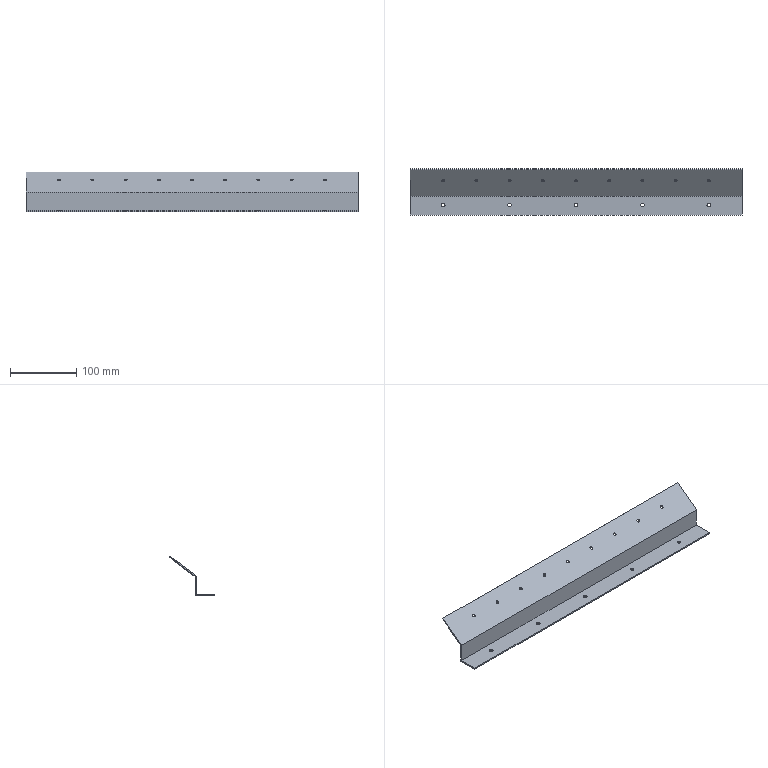Part | SolidWorks | features BaseBody 1 | 1 solid | 38 faces | box 500 x 69.2 x 60 mm | volume 106489 mm3 | cylinder 28 | plane 10 | commonest cylinder face diameters 4.4 x18 5.5 x10
STEP:
#1=CARTESIAN_POINT('',(546.946,-4176.013,1824.691));
#2=VERTEX_POINT('',#1);
#3=CARTESIAN_POINT('',(546.946,-4179.533,1822.051));
#4=VERTEX_POINT('',#3);
#5=CARTESIAN_POINT('',(546.946,-4177.773,1823.371));
#6=DIRECTION('',(0.,-0.6,0.8));
#7=DIRECTION('',(0.,-0.8,-0.6));
#8=AXIS2_PLACEMENT_3D('',#5,#6,#7);
#9=CIRCLE('',#8,2.2);
#10=EDGE_CURVE('',#2,#4,#9,.T.);
#11=ORIENTED_EDGE('',*,*,#10,.F.);
#12=CARTESIAN_POINT('',(546.946,-4177.213,1826.291));
#13=VERTEX_POINT('',#12);
#14=CARTESIAN_POINT('',(546.946,-4198.213,1854.291));
#15=DIRECTION('',(0.,-0.6,0.8));
#16=VECTOR('',#15,1000.);
#17=LINE('',#14,#16);
#18=EDGE_CURVE('',#2,#13,#17,.T.);
#19=ORIENTED_EDGE('',*,*,#18,.T.);
#20=CARTESIAN_POINT('',(546.946,-4180.733,1823.651));
#21=VERTEX_POINT('',#20);
#22=CARTESIAN_POINT('',(546.946,-4178.973,1824.971));
#23=DIRECTION('',(0.,0.6,-0.8));
#24=DIRECTION('',(0.,-0.8,-0.6));
#25=AXIS2_PLACEMENT_3D('',#22,#23,#24);
#26=CIRCLE('',#25,2.2);
#27=EDGE_CURVE('',#21,#13,#26,.T.);
#28=ORIENTED_EDGE('',*,*,#27,.F.);
#29=CARTESIAN_POINT('',(546.946,-4201.733,1851.651));
#30=DIRECTION('',(0.,-0.6,0.8));
#31=VECTOR('',#30,1000.);
#32=LINE('',#29,#31);
#33=EDGE_CURVE('',#4,#21,#32,.T.);
#34=ORIENTED_EDGE('',*,*,#33,.F.);
#35=EDGE_LOOP('',(#11,#19,#28,#34));
#36=FACE_OUTER_BOUND('',#35,.T.);
#37=CARTESIAN_POINT('',(546.946,-4199.973,1852.971));
#38=DIRECTION('',(0.,-0.6,0.8));
#39=DIRECTION('',(0.,-0.8,-0.6));
#40=AXIS2_PLACEMENT_3D('',#37,#38,#39);
#41=CYLINDRICAL_SURFACE('',#40,2.2);
#42=ADVANCED_FACE('',(#36),#41,.F.);
#43=CARTESIAN_POINT('',(446.946,-4176.013,1824.691));
#44=VERTEX_POINT('',#43);
#45=CARTESIAN_POINT('',(446.946,-4179.533,1822.051));
#46=VERTEX_POINT('',#45);
#47=CARTESIAN_POINT('',(446.946,-4177.773,1823.371));
#48=DIRECTION('',(0.,-0.6,0.8));
#49=DIRECTION('',(0.,-0.8,-0.6));
#50=AXIS2_PLACEMENT_3D('',#47,#48,#49);
#51=CIRCLE('',#50,2.2);
#52=EDGE_CURVE('',#44,#46,#51,.T.);
#53=ORIENTED_EDGE('',*,*,#52,.F.);
#54=CARTESIAN_POINT('',(446.946,-4177.213,1826.291));
#55=VERTEX_POINT('',#54);
#56=CARTESIAN_POINT('',(446.946,-4198.213,1854.291));
#57=DIRECTION('',(0.,-0.6,0.8));
#58=VECTOR('',#57,1000.);
#59=LINE('',#56,#58);
#60=EDGE_CURVE('',#44,#55,#59,.T.);
#61=ORIENTED_EDGE('',*,*,#60,.T.);
#62=CARTESIAN_POINT('',(446.946,-4180.733,1823.651));
#63=VERTEX_POINT('',#62);
#64=CARTESIAN_POINT('',(446.946,-4178.973,1824.971));
#65=DIRECTION('',(0.,0.6,-0.8));
#66=DIRECTION('',(0.,-0.8,-0.6));
#67=AXIS2_PLACEMENT_3D('',#64,#65,#66);
#68=CIRCLE('',#67,2.2);
#69=EDGE_CURVE('',#63,#55,#68,.T.);
#70=ORIENTED_EDGE('',*,*,#69,.F.);
#71=CARTESIAN_POINT('',(446.946,-4201.733,1851.651));
#72=DIRECTION('',(0.,-0.6,0.8));
#73=VECTOR('',#72,1000.);
#74=LINE('',#71,#73);
#75=EDGE_CURVE('',#46,#63,#74,.T.);
#76=ORIENTED_EDGE('',*,*,#75,.F.);
#77=EDGE_LOOP('',(#53,#61,#70,#76));
#78=FACE_OUTER_BOUND('',#77,.T.);
#79=CARTESIAN_POINT('',(446.946,-4199.973,1852.971));
#80=DIRECTION('',(0.,-0.6,0.8));
#81=DIRECTION('',(0.,-0.8,-0.6));
#82=AXIS2_PLACEMENT_3D('',#79,#80,#81);
#83=CYLINDRICAL_SURFACE('',#82,2.2);
#84=ADVANCED_FACE('',(#78),#83,.F.);
#85=CARTESIAN_POINT('',(346.946,-4176.013,1824.691));
#86=VERTEX_POINT('',#85);
#87=CARTESIAN_POINT('',(346.946,-4179.533,1822.051));
#88=VERTEX_POINT('',#87);
#89=CARTESIAN_POINT('',(346.946,-4177.773,1823.371));
#90=DIRECTION('',(0.,-0.6,0.8));
#91=DIRECTION('',(0.,-0.8,-0.6));
#92=AXIS2_PLACEMENT_3D('',#89,#90,#91);
#93=CIRCLE('',#92,2.2);
#94=EDGE_CURVE('',#86,#88,#93,.T.);
#95=ORIENTED_EDGE('',*,*,#94,.F.);
#96=CARTESIAN_POINT('',(346.946,-4177.213,1826.291));
#97=VERTEX_POINT('',#96);
#98=CARTESIAN_POINT('',(346.946,-4198.213,1854.291));
#99=DIRECTION('',(0.,-0.6,0.8));
#100=VECTOR('',#99,1000.);
#101=LINE('',#98,#100);
#102=EDGE_CURVE('',#86,#97,#101,.T.);
#103=ORIENTED_EDGE('',*,*,#102,.T.);
#104=CARTESIAN_POINT('',(346.946,-4180.733,1823.651));
#105=VERTEX_POINT('',#104);
#106=CARTESIAN_POINT('',(346.946,-4178.973,1824.971));
#107=DIRECTION('',(0.,0.6,-0.8));
#108=DIRECTION('',(0.,-0.8,-0.6));
#109=AXIS2_PLACEMENT_3D('',#106,#107,#108);
#110=CIRCLE('',#109,2.2);
#111=EDGE_CURVE('',#105,#97,#110,.T.);
#112=ORIENTED_EDGE('',*,*,#111,.F.);
#113=CARTESIAN_POINT('',(346.946,-4201.733,1851.651));
#114=DIRECTION('',(0.,-0.6,0.8));
#115=VECTOR('',#114,1000.);
#116=LINE('',#113,#115);
#117=EDGE_CURVE('',#88,#105,#116,.T.);
#118=ORIENTED_EDGE('',*,*,#117,.F.);
#119=EDGE_LOOP('',(#95,#103,#112,#118));
#120=FACE_OUTER_BOUND('',#119,.T.);
#121=CARTESIAN_POINT('',(346.946,-4199.973,1852.971));
#122=DIRECTION('',(0.,-0.6,0.8));
#123=DIRECTION('',(0.,-0.8,-0.6));
#124=AXIS2_PLACEMENT_3D('',#121,#122,#123);
#125=CYLINDRICAL_SURFACE('',#124,2.2);
#126=ADVANCED_FACE('',(#120),#125,.F.);
#127=CARTESIAN_POINT('',(646.946,-4176.013,1824.691));
#128=VERTEX_POINT('',#127);
#129=CARTESIAN_POINT('',(646.946,-4179.533,1822.051));
#130=VERTEX_POINT('',#129);
#131=CARTESIAN_POINT('',(646.946,-4177.773,1823.371));
#132=DIRECTION('',(0.,-0.6,0.8));
#133=DIRECTION('',(0.,-0.8,-0.6));
#134=AXIS2_PLACEMENT_3D('',#131,#132,#133);
#135=CIRCLE('',#134,2.2);
#136=EDGE_CURVE('',#128,#130,#135,.T.);
#137=ORIENTED_EDGE('',*,*,#136,.F.);
#138=CARTESIAN_POINT('',(646.946,-4177.213,1826.291));
#139=VERTEX_POINT('',#138);
#140=CARTESIAN_POINT('',(646.946,-4198.213,1854.291));
#141=DIRECTION('',(0.,-0.6,0.8));
#142=VECTOR('',#141,1000.);
#143=LINE('',#140,#142);
#144=EDGE_CURVE('',#128,#139,#143,.T.);
#145=ORIENTED_EDGE('',*,*,#144,.T.);
#146=CARTESIAN_POINT('',(646.946,-4180.733,1823.651));
#147=VERTEX_POINT('',#146);
#148=CARTESIAN_POINT('',(646.946,-4178.973,1824.971));
#149=DIRECTION('',(0.,0.6,-0.8));
#150=DIRECTION('',(0.,-0.8,-0.6));
#151=AXIS2_PLACEMENT_3D('',#148,#149,#150);
#152=CIRCLE('',#151,2.2);
#153=EDGE_CURVE('',#147,#139,#152,.T.);
#154=ORIENTED_EDGE('',*,*,#153,.F.);
#155=CARTESIAN_POINT('',(646.946,-4201.733,1851.651));
#156=DIRECTION('',(0.,-0.6,0.8));
#157=VECTOR('',#156,1000.);
#158=LINE('',#155,#157);
#159=EDGE_CURVE('',#130,#147,#158,.T.);
#160=ORIENTED_EDGE('',*,*,#159,.F.);
#161=EDGE_LOOP('',(#137,#145,#154,#160));
#162=FACE_OUTER_BOUND('',#161,.T.);
#163=CARTESIAN_POINT('',(646.946,-4199.973,1852.971));
#164=DIRECTION('',(0.,-0.6,0.8));
#165=DIRECTION('',(0.,-0.8,-0.6));
#166=AXIS2_PLACEMENT_3D('',#163,#164,#165);
#167=CYLINDRICAL_SURFACE('',#166,2.2);
#168=ADVANCED_FACE('',(#162),#167,.F.);
#169=CARTESIAN_POINT('',(746.946,-4176.013,1824.691));
#170=VERTEX_POINT('',#169);
#171=CARTESIAN_POINT('',(746.946,-4179.533,1822.051));
#172=VERTEX_POINT('',#171);
#173=CARTESIAN_POINT('',(746.946,-4177.773,1823.371));
#174=DIRECTION('',(0.,-0.6,0.8));
#175=DIRECTION('',(0.,-0.8,-0.6));
#176=AXIS2_PLACEMENT_3D('',#173,#174,#175);
#177=CIRCLE('',#176,2.2);
#178=EDGE_CURVE('',#170,#172,#177,.T.);
#179=ORIENTED_EDGE('',*,*,#178,.F.);
#180=CARTESIAN_POINT('',(746.946,-4177.213,1826.291));
#181=VERTEX_POINT('',#180);
#182=CARTESIAN_POINT('',(746.946,-4198.213,1854.291));
#183=DIRECTION('',(0.,-0.6,0.8));
#184=VECTOR('',#183,1000.);
#185=LINE('',#182,#184);
#186=EDGE_CURVE('',#170,#181,#185,.T.);
#187=ORIENTED_EDGE('',*,*,#186,.T.);
#188=CARTESIAN_POINT('',(746.946,-4180.733,1823.651));
#189=VERTEX_POINT('',#188);
#190=CARTESIAN_POINT('',(746.946,-4178.973,1824.971));
#191=DIRECTION('',(0.,0.6,-0.8));
#192=DIRECTION('',(0.,-0.8,-0.6));
#193=AXIS2_PLACEMENT_3D('',#190,#191,#192);
#194=CIRCLE('',#193,2.2);
#195=EDGE_CURVE('',#189,#181,#194,.T.);
#196=ORIENTED_EDGE('',*,*,#195,.F.);
#197=CARTESIAN_POINT('',(746.946,-4201.733,1851.651));
#198=DIRECTION('',(0.,-0.6,0.8));
#199=VECTOR('',#198,1000.);
#200=LINE('',#197,#199);
#201=EDGE_CURVE('',#172,#189,#200,.T.);
#202=ORIENTED_EDGE('',*,*,#201,.F.);
#203=EDGE_LOOP('',(#179,#187,#196,#202));
#204=FACE_OUTER_BOUND('',#203,.T.);
#205=CARTESIAN_POINT('',(746.946,-4199.973,1852.971));
#206=DIRECTION('',(0.,-0.6,0.8));
#207=DIRECTION('',(0.,-0.8,-0.6));
#208=AXIS2_PLACEMENT_3D('',#205,#206,#207);
#209=CYLINDRICAL_SURFACE('',#208,2.2);
#210=ADVANCED_FACE('',(#204),#209,.F.);
#211=CARTESIAN_POINT('',(596.946,-4176.013,1824.691));
#212=VERTEX_POINT('',#211);
#213=CARTESIAN_POINT('',(596.946,-4179.533,1822.051));
#214=VERTEX_POINT('',#213);
#215=CARTESIAN_POINT('',(596.946,-4177.773,1823.371));
#216=DIRECTION('',(0.,-0.6,0.8));
#217=DIRECTION('',(0.,-0.8,-0.6));
#218=AXIS2_PLACEMENT_3D('',#215,#216,#217);
#219=CIRCLE('',#218,2.2);
#220=EDGE_CURVE('',#212,#214,#219,.T.);
#221=ORIENTED_EDGE('',*,*,#220,.F.);
#222=CARTESIAN_POINT('',(596.946,-4177.213,1826.291));
#223=VERTEX_POINT('',#222);
#224=CARTESIAN_POINT('',(596.946,-4198.213,1854.291));
#225=DIRECTION('',(0.,-0.6,0.8));
#226=VECTOR('',#225,1000.);
#227=LINE('',#224,#226);
#228=EDGE_CURVE('',#212,#223,#227,.T.);
#229=ORIENTED_EDGE('',*,*,#228,.T.);
#230=CARTESIAN_POINT('',(596.946,-4180.733,1823.651));
#231=VERTEX_POINT('',#230);
#232=CARTESIAN_POINT('',(596.946,-4178.973,1824.971));
#233=DIRECTION('',(0.,0.6,-0.8));
#234=DIRECTION('',(0.,-0.8,-0.6));
#235=AXIS2_PLACEMENT_3D('',#232,#233,#234);
#236=CIRCLE('',#235,2.2);
#237=EDGE_CURVE('',#231,#223,#236,.T.);
#238=ORIENTED_EDGE('',*,*,#237,.F.);
#239=CARTESIAN_POINT('',(596.946,-4201.733,1851.651));
#240=DIRECTION('',(0.,-0.6,0.8));
#241=VECTOR('',#240,1000.);
#242=LINE('',#239,#241);
#243=EDGE_CURVE('',#214,#231,#242,.T.);
#244=ORIENTED_EDGE('',*,*,#243,.F.);
#245=EDGE_LOOP('',(#221,#229,#238,#244));
#246=FACE_OUTER_BOUND('',#245,.T.);
#247=CARTESIAN_POINT('',(596.946,-4199.973,1852.971));
#248=DIRECTION('',(0.,-0.6,0.8));
#249=DIRECTION('',(0.,-0.8,-0.6));
#250=AXIS2_PLACEMENT_3D('',#247,#248,#249);
#251=CYLINDRICAL_SURFACE('',#250,2.2);
#252=ADVANCED_FACE('',(#246),#251,.F.);
#253=CARTESIAN_POINT('',(696.946,-4176.013,1824.691));
#254=VERTEX_POINT('',#253);
#255=CARTESIAN_POINT('',(696.946,-4179.533,1822.051));
#256=VERTEX_POINT('',#255);
#257=CARTESIAN_POINT('',(696.946,-4177.773,1823.371));
#258=DIRECTION('',(0.,-0.6,0.8));
#259=DIRECTION('',(0.,-0.8,-0.6));
#260=AXIS2_PLACEMENT_3D('',#257,#258,#259);
#261=CIRCLE('',#260,2.2);
#262=EDGE_CURVE('',#254,#256,#261,.T.);
#263=ORIENTED_EDGE('',*,*,#262,.F.);
#264=CARTESIAN_POINT('',(696.946,-4177.213,1826.291));
#265=VERTEX_POINT('',#264);
#266=CARTESIAN_POINT('',(696.946,-4198.213,1854.291));
#267=DIRECTION('',(0.,-0.6,0.8));
#268=VECTOR('',#267,1000.);
#269=LINE('',#266,#268);
#270=EDGE_CURVE('',#254,#265,#269,.T.);
#271=ORIENTED_EDGE('',*,*,#270,.T.);
#272=CARTESIAN_POINT('',(696.946,-4180.733,1823.651));
#273=VERTEX_POINT('',#272);
#274=CARTESIAN_POINT('',(696.946,-4178.973,1824.971));
#275=DIRECTION('',(0.,0.6,-0.8));
#276=DIRECTION('',(0.,-0.8,-0.6));
#277=AXIS2_PLACEMENT_3D('',#274,#275,#276);
#278=CIRCLE('',#277,2.2);
#279=EDGE_CURVE('',#273,#265,#278,.T.);
#280=ORIENTED_EDGE('',*,*,#279,.F.);
#281=CARTESIAN_POINT('',(696.946,-4201.733,1851.651));
#282=DIRECTION('',(0.,-0.6,0.8));
#283=VECTOR('',#282,1000.);
#284=LINE('',#281,#283);
#285=EDGE_CURVE('',#256,#273,#284,.T.);
#286=ORIENTED_EDGE('',*,*,#285,.F.);
#287=EDGE_LOOP('',(#263,#271,#280,#286));
#288=FACE_OUTER_BOUND('',#287,.T.);
#289=CARTESIAN_POINT('',(696.946,-4199.973,1852.971));
#290=DIRECTION('',(0.,-0.6,0.8));
#291=DIRECTION('',(0.,-0.8,-0.6));
#292=AXIS2_PLACEMENT_3D('',#289,#290,#291);
#293=CYLINDRICAL_SURFACE('',#292,2.2);
#294=ADVANCED_FACE('',(#288),#293,.F.);
#295=CARTESIAN_POINT('',(396.946,-4176.013,1824.691));
#296=VERTEX_POINT('',#295);
#297=CARTESIAN_POINT('',(396.946,-4179.533,1822.051));
#298=VERTEX_POINT('',#297);
#299=CARTESIAN_POINT('',(396.946,-4177.773,1823.371));
#300=DIRECTION('',(0.,-0.6,0.8));
#301=DIRECTION('',(0.,-0.8,-0.6));
#302=AXIS2_PLACEMENT_3D('',#299,#300,#301);
#303=CIRCLE('',#302,2.2);
#304=EDGE_CURVE('',#296,#298,#303,.T.);
#305=ORIENTED_EDGE('',*,*,#304,.F.);
#306=CARTESIAN_POINT('',(396.946,-4177.213,1826.291));
#307=VERTEX_POINT('',#306);
#308=CARTESIAN_POINT('',(396.946,-4198.213,1854.291));
#309=DIRECTION('',(0.,-0.6,0.8));
#310=VECTOR('',#309,1000.);
#311=LINE('',#308,#310);
#312=EDGE_CURVE('',#296,#307,#311,.T.);
#313=ORIENTED_EDGE('',*,*,#312,.T.);
#314=CARTESIAN_POINT('',(396.946,-4180.733,1823.651));
#315=VERTEX_POINT('',#314);
#316=CARTESIAN_POINT('',(396.946,-4178.973,1824.971));
#317=DIRECTION('',(0.,0.6,-0.8));
#318=DIRECTION('',(0.,-0.8,-0.6));
#319=AXIS2_PLACEMENT_3D('',#316,#317,#318);
#320=CIRCLE('',#319,2.2);
#321=EDGE_CURVE('',#315,#307,#320,.T.);
#322=ORIENTED_EDGE('',*,*,#321,.F.);
#323=CARTESIAN_POINT('',(396.946,-4201.733,1851.651));
#324=DIRECTION('',(0.,-0.6,0.8));
#325=VECTOR('',#324,1000.);
#326=LINE('',#323,#325);
#327=EDGE_CURVE('',#298,#315,#326,.T.);
#328=ORIENTED_EDGE('',*,*,#327,.F.);
#329=EDGE_LOOP('',(#305,#313,#322,#328));
#330=FACE_OUTER_BOUND('',#329,.T.);
#331=CARTESIAN_POINT('',(396.946,-4199.973,1852.971));
#332=DIRECTION('',(0.,-0.6,0.8));
#333=DIRECTION('',(0.,-0.8,-0.6));
#334=AXIS2_PLACEMENT_3D('',#331,#332,#333);
#335=CYLINDRICAL_SURFACE('',#334,2.2);
#336=ADVANCED_FACE('',(#330),#335,.F.);
#337=CARTESIAN_POINT('',(496.946,-4176.013,1824.691));
#338=VERTEX_POINT('',#337);
#339=CARTESIAN_POINT('',(496.946,-4179.533,1822.051));
#340=VERTEX_POINT('',#339);
#341=CARTESIAN_POINT('',(496.946,-4177.773,1823.371));
#342=DIRECTION('',(0.,-0.6,0.8));
#343=DIRECTION('',(0.,-0.8,-0.6));
#344=AXIS2_PLACEMENT_3D('',#341,#342,#343);
#345=CIRCLE('',#344,2.2);
#346=EDGE_CURVE('',#338,#340,#345,.T.);
#347=ORIENTED_EDGE('',*,*,#346,.F.);
#348=CARTESIAN_POINT('',(496.946,-4177.213,1826.291));
#349=VERTEX_POINT('',#348);
#350=CARTESIAN_POINT('',(496.946,-4198.213,1854.291));
#351=DIRECTION('',(0.,-0.6,0.8));
#352=VECTOR('',#351,1000.);
#353=LINE('',#350,#352);
#354=EDGE_CURVE('',#338,#349,#353,.T.);
#355=ORIENTED_EDGE('',*,*,#354,.T.);
#356=CARTESIAN_POINT('',(496.946,-4180.733,1823.651));
#357=VERTEX_POINT('',#356);
#358=CARTESIAN_POINT('',(496.946,-4178.973,1824.971));
#359=DIRECTION('',(0.,0.6,-0.8));
#360=DIRECTION('',(0.,-0.8,-0.6));
#361=AXIS2_PLACEMENT_3D('',#358,#359,#360);
#362=CIRCLE('',#361,2.2);
#363=EDGE_CURVE('',#357,#349,#362,.T.);
#364=ORIENTED_EDGE('',*,*,#363,.F.);
#365=CARTESIAN_POINT('',(496.946,-4201.733,1851.651));
#366=DIRECTION('',(0.,-0.6,0.8));
#367=VECTOR('',#366,1000.);
#368=LINE('',#365,#367);
#369=EDGE_CURVE('',#340,#357,#368,.T.);
#370=ORIENTED_EDGE('',*,*,#369,.F.);
#371=EDGE_LOOP('',(#347,#355,#364,#370));
#372=FACE_OUTER_BOUND('',#371,.T.);
#373=CARTESIAN_POINT('',(496.946,-4199.973,1852.971));
#374=DIRECTION('',(0.,-0.6,0.8));
#375=DIRECTION('',(0.,-0.8,-0.6));
#376=AXIS2_PLACEMENT_3D('',#373,#374,#375);
#377=CYLINDRICAL_SURFACE('',#376,2.2);
#378=ADVANCED_FACE('',(#372),#377,.F.);
#379=CARTESIAN_POINT('',(444.196,-4215.973,1776.971));
#380=VERTEX_POINT('',#379);
#381=CARTESIAN_POINT('',(449.696,-4215.973,1776.971));
#382=VERTEX_POINT('',#381);
#383=CARTESIAN_POINT('',(446.946,-4215.973,1776.971));
#384=DIRECTION('',(0.,0.,1.));
#385=DIRECTION('',(1.,0.,0.));
#386=AXIS2_PLACEMENT_3D('',#383,#384,#385);
#387=CIRCLE('',#386,2.75);
#388=EDGE_CURVE('',#380,#382,#387,.T.);
#389=ORIENTED_EDGE('',*,*,#388,.F.);
#390=CARTESIAN_POINT('',(444.196,-4215.973,1778.971));
#391=VERTEX_POINT('',#390);
#392=CARTESIAN_POINT('',(444.196,-4215.973,1778.308));
#393=DIRECTION('',(0.,0.,1.));
#394=VECTOR('',#393,1000.);
#395=LINE('',#392,#394);
#396=EDGE_CURVE('',#380,#391,#395,.T.);
#397=ORIENTED_EDGE('',*,*,#396,.T.);
#398=CARTESIAN_POINT('',(449.696,-4215.973,1778.971));
#399=VERTEX_POINT('',#398);
#400=CARTESIAN_POINT('',(446.946,-4215.973,1778.971));
#401=DIRECTION('',(0.,0.,-1.));
#402=DIRECTION('',(1.,0.,0.));
#403=AXIS2_PLACEMENT_3D('',#400,#401,#402);
#404=CIRCLE('',#403,2.75);
#405=EDGE_CURVE('',#399,#391,#404,.T.);
#406=ORIENTED_EDGE('',*,*,#405,.F.);
#407=CARTESIAN_POINT('',(449.696,-4215.973,1778.308));
#408=DIRECTION('',(0.,0.,1.));
#409=VECTOR('',#408,1000.);
#410=LINE('',#407,#409);
#411=EDGE_CURVE('',#382,#399,#410,.T.);
#412=ORIENTED_EDGE('',*,*,#411,.F.);
#413=EDGE_LOOP('',(#389,#397,#406,#412));
#414=FACE_OUTER_BOUND('',#413,.T.);
#415=CARTESIAN_POINT('',(446.946,-4215.973,1778.308));
#416=DIRECTION('',(0.,0.,1.));
#417=DIRECTION('',(1.,0.,0.));
#418=AXIS2_PLACEMENT_3D('',#415,#416,#417);
#419=CYLINDRICAL_SURFACE('',#418,2.75);
#420=ADVANCED_FACE('',(#414),#419,.F.);
#421=CARTESIAN_POINT('',(549.696,-4215.973,1778.971));
#422=VERTEX_POINT('',#421);
#423=CARTESIAN_POINT('',(544.196,-4215.973,1778.971));
#424=VERTEX_POINT('',#423);
#425=CARTESIAN_POINT('',(546.946,-4215.973,1778.971));
#426=DIRECTION('',(0.,0.,-1.));
#427=DIRECTION('',(-1.,0.,0.));
#428=AXIS2_PLACEMENT_3D('',#425,#426,#427);
#429=CIRCLE('',#428,2.75);
#430=EDGE_CURVE('',#422,#424,#429,.T.);
#431=ORIENTED_EDGE('',*,*,#430,.F.);
#432=CARTESIAN_POINT('',(549.696,-4215.973,1776.971));
#433=VERTEX_POINT('',#432);
#434=CARTESIAN_POINT('',(549.696,-4215.973,1778.308));
#435=DIRECTION('',(0.,0.,-1.));
#436=VECTOR('',#435,1000.);
#437=LINE('',#434,#436);
#438=EDGE_CURVE('',#422,#433,#437,.T.);
#439=ORIENTED_EDGE('',*,*,#438,.T.);
#440=CARTESIAN_POINT('',(544.196,-4215.973,1776.971));
#441=VERTEX_POINT('',#440);
#442=CARTESIAN_POINT('',(546.946,-4215.973,1776.971));
#443=DIRECTION('',(0.,0.,1.));
#444=DIRECTION('',(-1.,0.,0.));
#445=AXIS2_PLACEMENT_3D('',#442,#443,#444);
#446=CIRCLE('',#445,2.75);
#447=EDGE_CURVE('',#441,#433,#446,.T.);
#448=ORIENTED_EDGE('',*,*,#447,.F.);
#449=CARTESIAN_POINT('',(544.196,-4215.973,1778.308));
#450=DIRECTION('',(0.,0.,-1.));
#451=VECTOR('',#450,1000.);
#452=LINE('',#449,#451);
#453=EDGE_CURVE('',#424,#441,#452,.T.);
#454=ORIENTED_EDGE('',*,*,#453,.F.);
#455=EDGE_LOOP('',(#431,#439,#448,#454));
#456=FACE_OUTER_BOUND('',#455,.T.);
#457=CARTESIAN_POINT('',(546.946,-4215.973,1778.308));
#458=DIRECTION('',(0.,0.,-1.));
#459=DIRECTION('',(-1.,0.,0.));
#460=AXIS2_PLACEMENT_3D('',#457,#458,#459);
#461=CYLINDRICAL_SURFACE('',#460,2.75);
#462=ADVANCED_FACE('',(#456),#461,.F.);
#463=CARTESIAN_POINT('',(749.696,-4215.973,1778.971));
#464=VERTEX_POINT('',#463);
#465=CARTESIAN_POINT('',(744.196,-4215.973,1778.971));
#466=VERTEX_POINT('',#465);
#467=CARTESIAN_POINT('',(746.946,-4215.973,1778.971));
#468=DIRECTION('',(0.,0.,-1.));
#469=DIRECTION('',(-1.,0.,0.));
#470=AXIS2_PLACEMENT_3D('',#467,#468,#469);
#471=CIRCLE('',#470,2.75);
#472=EDGE_CURVE('',#464,#466,#471,.T.);
#473=ORIENTED_EDGE('',*,*,#472,.F.);
#474=CARTESIAN_POINT('',(749.696,-4215.973,1776.971));
#475=VERTEX_POINT('',#474);
#476=CARTESIAN_POINT('',(749.696,-4215.973,1778.308));
#477=DIRECTION('',(0.,0.,-1.));
#478=VECTOR('',#477,1000.);
#479=LINE('',#476,#478);
#480=EDGE_CURVE('',#464,#475,#479,.T.);
#481=ORIENTED_EDGE('',*,*,#480,.T.);
#482=CARTESIAN_POINT('',(744.196,-4215.973,1776.971));
#483=VERTEX_POINT('',#482);
#484=CARTESIAN_POINT('',(746.946,-4215.973,1776.971));
#485=DIRECTION('',(0.,0.,1.));
#486=DIRECTION('',(-1.,0.,0.));
#487=AXIS2_PLACEMENT_3D('',#484,#485,#486);
#488=CIRCLE('',#487,2.75);
#489=EDGE_CURVE('',#483,#475,#488,.T.);
#490=ORIENTED_EDGE('',*,*,#489,.F.);
#491=CARTESIAN_POINT('',(744.196,-4215.973,1778.308));
#492=DIRECTION('',(0.,0.,-1.));
#493=VECTOR('',#492,1000.);
#494=LINE('',#491,#493);
#495=EDGE_CURVE('',#466,#483,#494,.T.);
#496=ORIENTED_EDGE('',*,*,#495,.F.);
#497=EDGE_LOOP('',(#473,#481,#490,#496));
#498=FACE_OUTER_BOUND('',#497,.T.);
#499=CARTESIAN_POINT('',(746.946,-4215.973,1778.308));
#500=DIRECTION('',(0.,0.,-1.));
#501=DIRECTION('',(-1.,0.,0.));
#502=AXIS2_PLACEMENT_3D('',#499,#500,#501);
#503=CYLINDRICAL_SURFACE('',#502,2.75);
#504=ADVANCED_FACE('',(#498),#503,.F.);
#505=CARTESIAN_POINT('',(649.696,-4215.973,1778.971));
#506=VERTEX_POINT('',#505);
#507=CARTESIAN_POINT('',(644.196,-4215.973,1778.971));
#508=VERTEX_POINT('',#507);
#509=CARTESIAN_POINT('',(646.946,-4215.973,1778.971));
#510=DIRECTION('',(0.,0.,-1.));
#511=DIRECTION('',(-1.,0.,0.));
#512=AXIS2_PLACEMENT_3D('',#509,#510,#511);
#513=CIRCLE('',#512,2.75);
#514=EDGE_CURVE('',#506,#508,#513,.T.);
#515=ORIENTED_EDGE('',*,*,#514,.F.);
#516=CARTESIAN_POINT('',(649.696,-4215.973,1776.971));
#517=VERTEX_POINT('',#516);
#518=CARTESIAN_POINT('',(649.696,-4215.973,1778.308));
#519=DIRECTION('',(0.,0.,-1.));
#520=VECTOR('',#519,1000.);
#521=LINE('',#518,#520);
#522=EDGE_CURVE('',#506,#517,#521,.T.);
#523=ORIENTED_EDGE('',*,*,#522,.T.);
#524=CARTESIAN_POINT('',(644.196,-4215.973,1776.971));
#525=VERTEX_POINT('',#524);
#526=CARTESIAN_POINT('',(646.946,-4215.973,1776.971));
#527=DIRECTION('',(0.,0.,1.));
#528=DIRECTION('',(-1.,0.,0.));
#529=AXIS2_PLACEMENT_3D('',#526,#527,#528);
#530=CIRCLE('',#529,2.75);
#531=EDGE_CURVE('',#525,#517,#530,.T.);
#532=ORIENTED_EDGE('',*,*,#531,.F.);
#533=CARTESIAN_POINT('',(644.196,-4215.973,1778.308));
#534=DIRECTION('',(0.,0.,-1.));
#535=VECTOR('',#534,1000.);
#536=LINE('',#533,#535);
#537=EDGE_CURVE('',#508,#525,#536,.T.);
#538=ORIENTED_EDGE('',*,*,#537,.F.);
#539=EDGE_LOOP('',(#515,#523,#532,#538));
#540=FACE_OUTER_BOUND('',#539,.T.);
#541=CARTESIAN_POINT('',(646.946,-4215.973,1778.308));
#542=DIRECTION('',(0.,0.,-1.));
#543=DIRECTION('',(-1.,0.,0.));
#544=AXIS2_PLACEMENT_3D('',#541,#542,#543);
#545=CYLINDRICAL_SURFACE('',#544,2.75);
#546=ADVANCED_FACE('',(#540),#545,.F.);
#547=CARTESIAN_POINT('',(344.196,-4215.973,1776.971));
#548=VERTEX_POINT('',#547);
#549=CARTESIAN_POINT('',(349.696,-4215.973,1776.971));
#550=VERTEX_POINT('',#549);
#551=CARTESIAN_POINT('',(346.946,-4215.973,1776.971));
#552=DIRECTION('',(0.,0.,1.));
#553=DIRECTION('',(1.,0.,0.));
#554=AXIS2_PLACEMENT_3D('',#551,#552,#553);
#555=CIRCLE('',#554,2.75);
#556=EDGE_CURVE('',#548,#550,#555,.T.);
#557=ORIENTED_EDGE('',*,*,#556,.F.);
#558=CARTESIAN_POINT('',(344.196,-4215.973,1778.971));
#559=VERTEX_POINT('',#558);
#560=CARTESIAN_POINT('',(344.196,-4215.973,1778.308));
#561=DIRECTION('',(0.,0.,1.));
#562=VECTOR('',#561,1000.);
#563=LINE('',#560,#562);
#564=EDGE_CURVE('',#548,#559,#563,.T.);
#565=ORIENTED_EDGE('',*,*,#564,.T.);
#566=CARTESIAN_POINT('',(349.696,-4215.973,1778.971));
#567=VERTEX_POINT('',#566);
#568=CARTESIAN_POINT('',(346.946,-4215.973,1778.971));
#569=DIRECTION('',(0.,0.,-1.));
#570=DIRECTION('',(1.,0.,0.));
#571=AXIS2_PLACEMENT_3D('',#568,#569,#570);
#572=CIRCLE('',#571,2.75);
#573=EDGE_CURVE('',#567,#559,#572,.T.);
#574=ORIENTED_EDGE('',*,*,#573,.F.);
#575=CARTESIAN_POINT('',(349.696,-4215.973,1778.308));
#576=DIRECTION('',(0.,0.,1.));
#577=VECTOR('',#576,1000.);
#578=LINE('',#575,#577);
#579=EDGE_CURVE('',#550,#567,#578,.T.);
#580=ORIENTED_EDGE('',*,*,#579,.F.);
#581=EDGE_LOOP('',(#557,#565,#574,#580));
#582=FACE_OUTER_BOUND('',#581,.T.);
#583=CARTESIAN_POINT('',(346.946,-4215.973,1778.308));
#584=DIRECTION('',(0.,0.,1.));
#585=DIRECTION('',(1.,0.,0.));
#586=AXIS2_PLACEMENT_3D('',#583,#584,#585);
#587=CYLINDRICAL_SURFACE('',#586,2.75);
#588=ADVANCED_FACE('',(#582),#587,.F.);
#589=CARTESIAN_POINT('',(796.946,-4202.973,1806.971));
#590=VERTEX_POINT('',#589);
#591=CARTESIAN_POINT('',(796.946,-4162.973,1836.971));
#592=VERTEX_POINT('',#591);
#593=CARTESIAN_POINT('',(796.946,-4162.973,1836.971));
#594=DIRECTION('',(0.,0.8,0.6));
#595=VECTOR('',#594,1000.);
#596=LINE('',#593,#595);
#597=EDGE_CURVE('',#590,#592,#596,.T.);
#598=ORIENTED_EDGE('',*,*,#597,.T.);
#599=CARTESIAN_POINT('',(296.946,-4162.973,1836.971));
#600=VERTEX_POINT('',#599);
#601=CARTESIAN_POINT('',(796.946,-4162.973,1836.971));
#602=DIRECTION('',(-1.,0.,0.));
#603=VECTOR('',#602,1000.);
#604=LINE('',#601,#603);
#605=EDGE_CURVE('',#592,#600,#604,.T.);
#606=ORIENTED_EDGE('',*,*,#605,.T.);
#607=CARTESIAN_POINT('',(296.946,-4202.973,1806.971));
#608=VERTEX_POINT('',#607);
#609=CARTESIAN_POINT('',(296.946,-4162.973,1836.971));
#610=DIRECTION('',(0.,-0.8,-0.6));
#611=VECTOR('',#610,1000.);
#612=LINE('',#609,#611);
#613=EDGE_CURVE('',#600,#608,#612,.T.);
#614=ORIENTED_EDGE('',*,*,#613,.T.);
#615=CARTESIAN_POINT('',(796.946,-4202.973,1806.971));
#616=DIRECTION('',(1.,0.,0.));
#617=VECTOR('',#616,1000.);
#618=LINE('',#615,#617);
#619=EDGE_CURVE('',#608,#590,#618,.T.);
#620=ORIENTED_EDGE('',*,*,#619,.T.);
#621=EDGE_LOOP('',(#598,#606,#614,#620));
#622=FACE_OUTER_BOUND('',#621,.T.);
#623=ORIENTED_EDGE('',*,*,#27,.T.);
#624=CARTESIAN_POINT('',(546.946,-4178.973,1824.971));
#625=DIRECTION('',(0.,0.6,-0.8));
#626=DIRECTION('',(0.,-0.8,-0.6));
#627=AXIS2_PLACEMENT_3D('',#624,#625,#626);
#628=CIRCLE('',#627,2.2);
#629=EDGE_CURVE('',#13,#21,#628,.T.);
#630=ORIENTED_EDGE('',*,*,#629,.T.);
#631=EDGE_LOOP('',(#623,#630));
#632=FACE_BOUND('',#631,.T.);
#633=ORIENTED_EDGE('',*,*,#69,.T.);
#634=CARTESIAN_POINT('',(446.946,-4178.973,1824.971));
#635=DIRECTION('',(0.,0.6,-0.8));
#636=DIRECTION('',(0.,-0.8,-0.6));
#637=AXIS2_PLACEMENT_3D('',#634,#635,#636);
#638=CIRCLE('',#637,2.2);
#639=EDGE_CURVE('',#55,#63,#638,.T.);
#640=ORIENTED_EDGE('',*,*,#639,.T.);
#641=EDGE_LOOP('',(#633,#640));
#642=FACE_BOUND('',#641,.T.);
#643=ORIENTED_EDGE('',*,*,#111,.T.);
#644=CARTESIAN_POINT('',(346.946,-4178.973,1824.971));
#645=DIRECTION('',(0.,0.6,-0.8));
#646=DIRECTION('',(0.,-0.8,-0.6));
#647=AXIS2_PLACEMENT_3D('',#644,#645,#646);
#648=CIRCLE('',#647,2.2);
#649=EDGE_CURVE('',#97,#105,#648,.T.);
#650=ORIENTED_EDGE('',*,*,#649,.T.);
#651=EDGE_LOOP('',(#643,#650));
#652=FACE_BOUND('',#651,.T.);
#653=ORIENTED_EDGE('',*,*,#153,.T.);
#654=CARTESIAN_POINT('',(646.946,-4178.973,1824.971));
#655=DIRECTION('',(0.,0.6,-0.8));
#656=DIRECTION('',(0.,-0.8,-0.6));
#657=AXIS2_PLACEMENT_3D('',#654,#655,#656);
#658=CIRCLE('',#657,2.2);
#659=EDGE_CURVE('',#139,#147,#658,.T.);
#660=ORIENTED_EDGE('',*,*,#659,.T.);
#661=EDGE_LOOP('',(#653,#660));
#662=FACE_BOUND('',#661,.T.);
#663=ORIENTED_EDGE('',*,*,#195,.T.);
#664=CARTESIAN_POINT('',(746.946,-4178.973,1824.971));
#665=DIRECTION('',(0.,0.6,-0.8));
#666=DIRECTION('',(0.,-0.8,-0.6));
#667=AXIS2_PLACEMENT_3D('',#664,#665,#666);
#668=CIRCLE('',#667,2.2);
#669=EDGE_CURVE('',#181,#189,#668,.T.);
#670=ORIENTED_EDGE('',*,*,#669,.T.);
#671=EDGE_LOOP('',(#663,#670));
#672=FACE_BOUND('',#671,.T.);
#673=ORIENTED_EDGE('',*,*,#237,.T.);
#674=CARTESIAN_POINT('',(596.946,-4178.973,1824.971));
#675=DIRECTION('',(0.,0.6,-0.8));
#676=DIRECTION('',(0.,-0.8,-0.6));
#677=AXIS2_PLACEMENT_3D('',#674,#675,#676);
#678=CIRCLE('',#677,2.2);
#679=EDGE_CURVE('',#223,#231,#678,.T.);
#680=ORIENTED_EDGE('',*,*,#679,.T.);
#681=EDGE_LOOP('',(#673,#680));
#682=FACE_BOUND('',#681,.T.);
#683=ORIENTED_EDGE('',*,*,#279,.T.);
#684=CARTESIAN_POINT('',(696.946,-4178.973,1824.971));
#685=DIRECTION('',(0.,0.6,-0.8));
#686=DIRECTION('',(0.,-0.8,-0.6));
#687=AXIS2_PLACEMENT_3D('',#684,#685,#686);
#688=CIRCLE('',#687,2.2);
#689=EDGE_CURVE('',#265,#273,#688,.T.);
#690=ORIENTED_EDGE('',*,*,#689,.T.);
#691=EDGE_LOOP('',(#683,#690));
#692=FACE_BOUND('',#691,.T.);
#693=ORIENTED_EDGE('',*,*,#321,.T.);
#694=CARTESIAN_POINT('',(396.946,-4178.973,1824.971));
#695=DIRECTION('',(0.,0.6,-0.8));
#696=DIRECTION('',(0.,-0.8,-0.6));
#697=AXIS2_PLACEMENT_3D('',#694,#695,#696);
#698=CIRCLE('',#697,2.2);
#699=EDGE_CURVE('',#307,#315,#698,.T.);
#700=ORIENTED_EDGE('',*,*,#699,.T.);
#701=EDGE_LOOP('',(#693,#700));
#702=FACE_BOUND('',#701,.T.);
#703=ORIENTED_EDGE('',*,*,#363,.T.);
#704=CARTESIAN_POINT('',(496.946,-4178.973,1824.971));
#705=DIRECTION('',(0.,0.6,-0.8));
#706=DIRECTION('',(0.,-0.8,-0.6));
#707=AXIS2_PLACEMENT_3D('',#704,#705,#706);
#708=CIRCLE('',#707,2.2);
#709=EDGE_CURVE('',#349,#357,#708,.T.);
#710=ORIENTED_EDGE('',*,*,#709,.T.);
#711=EDGE_LOOP('',(#703,#710));
#712=FACE_BOUND('',#711,.T.);
#713=CARTESIAN_POINT('',(796.946,-4162.973,1836.971));
#714=DIRECTION('',(0.,-0.6,0.8));
#715=DIRECTION('',(0.,-0.8,-0.6));
#716=AXIS2_PLACEMENT_3D('',#713,#714,#715);
#717=PLANE('',#716);
#718=ADVANCED_FACE('',(#622,#632,#642,#652,#662,#672,#682,#692,#702,#712),#717,.T.);
#719=CARTESIAN_POINT('',(796.946,-4161.773,1835.371));
#720=VERTEX_POINT('',#719);
#721=CARTESIAN_POINT('',(796.946,-4161.773,1835.371));
#722=DIRECTION('',(0.,0.6,-0.8));
#723=VECTOR('',#722,1000.);
#724=LINE('',#721,#723);
#725=EDGE_CURVE('',#592,#720,#724,.T.);
#726=ORIENTED_EDGE('',*,*,#725,.T.);
#727=CARTESIAN_POINT('',(296.946,-4161.773,1835.371));
#728=VERTEX_POINT('',#727);
#729=CARTESIAN_POINT('',(796.946,-4161.773,1835.371));
#730=DIRECTION('',(-1.,0.,0.));
#731=VECTOR('',#730,1000.);
#732=LINE('',#729,#731);
#733=EDGE_CURVE('',#720,#728,#732,.T.);
#734=ORIENTED_EDGE('',*,*,#733,.T.);
#735=CARTESIAN_POINT('',(296.946,-4161.773,1835.371));
#736=DIRECTION('',(0.,-0.6,0.8));
#737=VECTOR('',#736,1000.);
#738=LINE('',#735,#737);
#739=EDGE_CURVE('',#728,#600,#738,.T.);
#740=ORIENTED_EDGE('',*,*,#739,.T.);
#741=ORIENTED_EDGE('',*,*,#605,.F.);
#742=EDGE_LOOP('',(#726,#734,#740,#741));
#743=FACE_OUTER_BOUND('',#742,.T.);
#744=CARTESIAN_POINT('',(796.946,-4161.773,1835.371));
#745=DIRECTION('',(0.,0.8,0.6));
#746=DIRECTION('',(0.,-0.6,0.8));
#747=AXIS2_PLACEMENT_3D('',#744,#745,#746);
#748=PLANE('',#747);
#749=ADVANCED_FACE('',(#743),#748,.T.);
#750=CARTESIAN_POINT('',(796.946,-4200.973,1776.971));
#751=VERTEX_POINT('',#750);
#752=CARTESIAN_POINT('',(796.946,-4200.973,1805.971));
#753=VERTEX_POINT('',#752);
#754=CARTESIAN_POINT('',(796.946,-4200.973,1801.908));
#755=DIRECTION('',(0.,0.,1.));
#756=VECTOR('',#755,1000.);
#757=LINE('',#754,#756);
#758=EDGE_CURVE('',#751,#753,#757,.T.);
#759=ORIENTED_EDGE('',*,*,#758,.T.);
#760=CARTESIAN_POINT('',(796.946,-4200.973,1805.971));
#761=DIRECTION('',(0.,0.8,0.6));
#762=VECTOR('',#761,1000.);
#763=LINE('',#760,#762);
#764=EDGE_CURVE('',#753,#720,#763,.T.);
#765=ORIENTED_EDGE('',*,*,#764,.T.);
#766=ORIENTED_EDGE('',*,*,#725,.F.);
#767=ORIENTED_EDGE('',*,*,#597,.F.);
#768=CARTESIAN_POINT('',(796.946,-4202.973,1778.971));
#769=VERTEX_POINT('',#768);
#770=CARTESIAN_POINT('',(796.946,-4202.973,1801.908));
#771=DIRECTION('',(0.,0.,-1.));
#772=VECTOR('',#771,1000.);
#773=LINE('',#770,#772);
#774=EDGE_CURVE('',#590,#769,#773,.T.);
#775=ORIENTED_EDGE('',*,*,#774,.T.);
#776=CARTESIAN_POINT('',(796.946,-4230.973,1778.971));
#777=VERTEX_POINT('',#776);
#778=CARTESIAN_POINT('',(796.946,-4196.736,1778.971));
#779=DIRECTION('',(0.,-1.,0.));
#780=VECTOR('',#779,1000.);
#781=LINE('',#778,#780);
#782=EDGE_CURVE('',#769,#777,#781,.T.);
#783=ORIENTED_EDGE('',*,*,#782,.T.);
#784=CARTESIAN_POINT('',(796.946,-4230.973,1776.971));
#785=VERTEX_POINT('',#784);
#786=CARTESIAN_POINT('',(796.946,-4230.973,1801.908));
#787=DIRECTION('',(0.,0.,-1.));
#788=VECTOR('',#787,1000.);
#789=LINE('',#786,#788);
#790=EDGE_CURVE('',#777,#785,#789,.T.);
#791=ORIENTED_EDGE('',*,*,#790,.T.);
#792=CARTESIAN_POINT('',(796.946,-4196.736,1776.971));
#793=DIRECTION('',(0.,1.,0.));
#794=VECTOR('',#793,1000.);
#795=LINE('',#792,#794);
#796=EDGE_CURVE('',#785,#751,#795,.T.);
#797=ORIENTED_EDGE('',*,*,#796,.T.);
#798=EDGE_LOOP('',(#759,#765,#766,#767,#775,#783,#791,#797));
#799=FACE_OUTER_BOUND('',#798,.T.);
#800=CARTESIAN_POINT('',(796.946,-4196.736,1801.908));
#801=DIRECTION('',(1.,0.,0.));
#802=DIRECTION('',(0.,0.,-1.));
#803=AXIS2_PLACEMENT_3D('',#800,#801,#802);
#804=PLANE('',#803);
#805=ADVANCED_FACE('',(#799),#804,.T.);
#806=ORIENTED_EDGE('',*,*,#774,.F.);
#807=ORIENTED_EDGE('',*,*,#619,.F.);
#808=CARTESIAN_POINT('',(296.946,-4202.973,1778.971));
#809=VERTEX_POINT('',#808);
#810=CARTESIAN_POINT('',(296.946,-4202.973,1806.971));
#811=DIRECTION('',(0.,0.,-1.));
#812=VECTOR('',#811,1000.);
#813=LINE('',#810,#812);
#814=EDGE_CURVE('',#608,#809,#813,.T.);
#815=ORIENTED_EDGE('',*,*,#814,.T.);
#816=CARTESIAN_POINT('',(796.946,-4202.973,1778.971));
#817=DIRECTION('',(1.,0.,0.));
#818=VECTOR('',#817,1000.);
#819=LINE('',#816,#818);
#820=EDGE_CURVE('',#809,#769,#819,.T.);
#821=ORIENTED_EDGE('',*,*,#820,.T.);
#822=EDGE_LOOP('',(#806,#807,#815,#821));
#823=FACE_OUTER_BOUND('',#822,.T.);
#824=CARTESIAN_POINT('',(796.946,-4202.973,1806.971));
#825=DIRECTION('',(0.,-1.,0.));
#826=DIRECTION('',(0.,0.,-1.));
#827=AXIS2_PLACEMENT_3D('',#824,#825,#826);
#828=PLANE('',#827);
#829=ADVANCED_FACE('',(#823),#828,.T.);
#830=ORIENTED_EDGE('',*,*,#739,.F.);
#831=CARTESIAN_POINT('',(296.946,-4200.973,1805.971));
#832=VERTEX_POINT('',#831);
#833=CARTESIAN_POINT('',(296.946,-4200.973,1805.971));
#834=DIRECTION('',(0.,0.8,0.6));
#835=VECTOR('',#834,1000.);
#836=LINE('',#833,#835);
#837=EDGE_CURVE('',#832,#728,#836,.T.);
#838=ORIENTED_EDGE('',*,*,#837,.F.);
#839=CARTESIAN_POINT('',(296.946,-4200.973,1776.971));
#840=VERTEX_POINT('',#839);
#841=CARTESIAN_POINT('',(296.946,-4200.973,1801.908));
#842=DIRECTION('',(0.,0.,1.));
#843=VECTOR('',#842,1000.);
#844=LINE('',#841,#843);
#845=EDGE_CURVE('',#840,#832,#844,.T.);
#846=ORIENTED_EDGE('',*,*,#845,.F.);
#847=CARTESIAN_POINT('',(296.946,-4230.973,1776.971));
#848=VERTEX_POINT('',#847);
#849=CARTESIAN_POINT('',(296.946,-4196.736,1776.971));
#850=DIRECTION('',(0.,1.,0.));
#851=VECTOR('',#850,1000.);
#852=LINE('',#849,#851);
#853=EDGE_CURVE('',#848,#840,#852,.T.);
#854=ORIENTED_EDGE('',*,*,#853,.F.);
#855=CARTESIAN_POINT('',(296.946,-4230.973,1778.971));
#856=VERTEX_POINT('',#855);
#857=CARTESIAN_POINT('',(296.946,-4230.973,1801.908));
#858=DIRECTION('',(0.,0.,-1.));
#859=VECTOR('',#858,1000.);
#860=LINE('',#857,#859);
#861=EDGE_CURVE('',#856,#848,#860,.T.);
#862=ORIENTED_EDGE('',*,*,#861,.F.);
#863=CARTESIAN_POINT('',(296.946,-4196.736,1778.971));
#864=DIRECTION('',(0.,-1.,0.));
#865=VECTOR('',#864,1000.);
#866=LINE('',#863,#865);
#867=EDGE_CURVE('',#809,#856,#866,.T.);
#868=ORIENTED_EDGE('',*,*,#867,.F.);
#869=ORIENTED_EDGE('',*,*,#814,.F.);
#870=ORIENTED_EDGE('',*,*,#613,.F.);
#871=EDGE_LOOP('',(#830,#838,#846,#854,#862,#868,#869,#870));
#872=FACE_OUTER_BOUND('',#871,.T.);
#873=CARTESIAN_POINT('',(296.946,-4196.736,1801.908));
#874=DIRECTION('',(1.,0.,0.));
#875=DIRECTION('',(0.,0.,-1.));
#876=AXIS2_PLACEMENT_3D('',#873,#874,#875);
#877=PLANE('',#876);
#878=ADVANCED_FACE('',(#872),#877,.F.);
#879=ORIENTED_EDGE('',*,*,#18,.F.);
#880=CARTESIAN_POINT('',(546.946,-4177.773,1823.371));
#881=DIRECTION('',(0.,-0.6,0.8));
#882=DIRECTION('',(0.,-0.8,-0.6));
#883=AXIS2_PLACEMENT_3D('',#880,#881,#882);
#884=CIRCLE('',#883,2.2);
#885=EDGE_CURVE('',#4,#2,#884,.T.);
#886=ORIENTED_EDGE('',*,*,#885,.F.);
#887=ORIENTED_EDGE('',*,*,#33,.T.);
#888=ORIENTED_EDGE('',*,*,#629,.F.);
#889=EDGE_LOOP('',(#879,#886,#887,#888));
#890=FACE_OUTER_BOUND('',#889,.T.);
#891=CARTESIAN_POINT('',(546.946,-4199.973,1852.971));
#892=DIRECTION('',(0.,-0.6,0.8));
#893=DIRECTION('',(0.,-0.8,-0.6));
#894=AXIS2_PLACEMENT_3D('',#891,#892,#893);
#895=CYLINDRICAL_SURFACE('',#894,2.2);
#896=ADVANCED_FACE('',(#890),#895,.F.);
#897=ORIENTED_EDGE('',*,*,#60,.F.);
#898=CARTESIAN_POINT('',(446.946,-4177.773,1823.371));
#899=DIRECTION('',(0.,-0.6,0.8));
#900=DIRECTION('',(0.,-0.8,-0.6));
#901=AXIS2_PLACEMENT_3D('',#898,#899,#900);
#902=CIRCLE('',#901,2.2);
#903=EDGE_CURVE('',#46,#44,#902,.T.);
#904=ORIENTED_EDGE('',*,*,#903,.F.);
#905=ORIENTED_EDGE('',*,*,#75,.T.);
#906=ORIENTED_EDGE('',*,*,#639,.F.);
#907=EDGE_LOOP('',(#897,#904,#905,#906));
#908=FACE_OUTER_BOUND('',#907,.T.);
#909=CARTESIAN_POINT('',(446.946,-4199.973,1852.971));
#910=DIRECTION('',(0.,-0.6,0.8));
#911=DIRECTION('',(0.,-0.8,-0.6));
#912=AXIS2_PLACEMENT_3D('',#909,#910,#911);
#913=CYLINDRICAL_SURFACE('',#912,2.2);
#914=ADVANCED_FACE('',(#908),#913,.F.);
#915=ORIENTED_EDGE('',*,*,#102,.F.);
#916=CARTESIAN_POINT('',(346.946,-4177.773,1823.371));
#917=DIRECTION('',(0.,-0.6,0.8));
#918=DIRECTION('',(0.,-0.8,-0.6));
#919=AXIS2_PLACEMENT_3D('',#916,#917,#918);
#920=CIRCLE('',#919,2.2);
#921=EDGE_CURVE('',#88,#86,#920,.T.);
#922=ORIENTED_EDGE('',*,*,#921,.F.);
#923=ORIENTED_EDGE('',*,*,#117,.T.);
#924=ORIENTED_EDGE('',*,*,#649,.F.);
#925=EDGE_LOOP('',(#915,#922,#923,#924));
#926=FACE_OUTER_BOUND('',#925,.T.);
#927=CARTESIAN_POINT('',(346.946,-4199.973,1852.971));
#928=DIRECTION('',(0.,-0.6,0.8));
#929=DIRECTION('',(0.,-0.8,-0.6));
#930=AXIS2_PLACEMENT_3D('',#927,#928,#929);
#931=CYLINDRICAL_SURFACE('',#930,2.2);
#932=ADVANCED_FACE('',(#926),#931,.F.);
#933=ORIENTED_EDGE('',*,*,#144,.F.);
#934=CARTESIAN_POINT('',(646.946,-4177.773,1823.371));
#935=DIRECTION('',(0.,-0.6,0.8));
#936=DIRECTION('',(0.,-0.8,-0.6));
#937=AXIS2_PLACEMENT_3D('',#934,#935,#936);
#938=CIRCLE('',#937,2.2);
#939=EDGE_CURVE('',#130,#128,#938,.T.);
#940=ORIENTED_EDGE('',*,*,#939,.F.);
#941=ORIENTED_EDGE('',*,*,#159,.T.);
#942=ORIENTED_EDGE('',*,*,#659,.F.);
#943=EDGE_LOOP('',(#933,#940,#941,#942));
#944=FACE_OUTER_BOUND('',#943,.T.);
#945=CARTESIAN_POINT('',(646.946,-4199.973,1852.971));
#946=DIRECTION('',(0.,-0.6,0.8));
#947=DIRECTION('',(0.,-0.8,-0.6));
#948=AXIS2_PLACEMENT_3D('',#945,#946,#947);
#949=CYLINDRICAL_SURFACE('',#948,2.2);
#950=ADVANCED_FACE('',(#944),#949,.F.);
#951=ORIENTED_EDGE('',*,*,#186,.F.);
#952=CARTESIAN_POINT('',(746.946,-4177.773,1823.371));
#953=DIRECTION('',(0.,-0.6,0.8));
#954=DIRECTION('',(0.,-0.8,-0.6));
#955=AXIS2_PLACEMENT_3D('',#952,#953,#954);
#956=CIRCLE('',#955,2.2);
#957=EDGE_CURVE('',#172,#170,#956,.T.);
#958=ORIENTED_EDGE('',*,*,#957,.F.);
#959=ORIENTED_EDGE('',*,*,#201,.T.);
#960=ORIENTED_EDGE('',*,*,#669,.F.);
#961=EDGE_LOOP('',(#951,#958,#959,#960));
#962=FACE_OUTER_BOUND('',#961,.T.);
#963=CARTESIAN_POINT('',(746.946,-4199.973,1852.971));
#964=DIRECTION('',(0.,-0.6,0.8));
#965=DIRECTION('',(0.,-0.8,-0.6));
#966=AXIS2_PLACEMENT_3D('',#963,#964,#965);
#967=CYLINDRICAL_SURFACE('',#966,2.2);
#968=ADVANCED_FACE('',(#962),#967,.F.);
#969=ORIENTED_EDGE('',*,*,#228,.F.);
#970=CARTESIAN_POINT('',(596.946,-4177.773,1823.371));
#971=DIRECTION('',(0.,-0.6,0.8));
#972=DIRECTION('',(0.,-0.8,-0.6));
#973=AXIS2_PLACEMENT_3D('',#970,#971,#972);
#974=CIRCLE('',#973,2.2);
#975=EDGE_CURVE('',#214,#212,#974,.T.);
#976=ORIENTED_EDGE('',*,*,#975,.F.);
#977=ORIENTED_EDGE('',*,*,#243,.T.);
#978=ORIENTED_EDGE('',*,*,#679,.F.);
#979=EDGE_LOOP('',(#969,#976,#977,#978));
#980=FACE_OUTER_BOUND('',#979,.T.);
#981=CARTESIAN_POINT('',(596.946,-4199.973,1852.971));
#982=DIRECTION('',(0.,-0.6,0.8));
#983=DIRECTION('',(0.,-0.8,-0.6));
#984=AXIS2_PLACEMENT_3D('',#981,#982,#983);
#985=CYLINDRICAL_SURFACE('',#984,2.2);
#986=ADVANCED_FACE('',(#980),#985,.F.);
#987=ORIENTED_EDGE('',*,*,#270,.F.);
#988=CARTESIAN_POINT('',(696.946,-4177.773,1823.371));
#989=DIRECTION('',(0.,-0.6,0.8));
#990=DIRECTION('',(0.,-0.8,-0.6));
#991=AXIS2_PLACEMENT_3D('',#988,#989,#990);
#992=CIRCLE('',#991,2.2);
#993=EDGE_CURVE('',#256,#254,#992,.T.);
#994=ORIENTED_EDGE('',*,*,#993,.F.);
#995=ORIENTED_EDGE('',*,*,#285,.T.);
#996=ORIENTED_EDGE('',*,*,#689,.F.);
#997=EDGE_LOOP('',(#987,#994,#995,#996));
#998=FACE_OUTER_BOUND('',#997,.T.);
#999=CARTESIAN_POINT('',(696.946,-4199.973,1852.971));
#1000=DIRECTION('',(0.,-0.6,0.8));
#1001=DIRECTION('',(0.,-0.8,-0.6));
#1002=AXIS2_PLACEMENT_3D('',#999,#1000,#1001);
#1003=CYLINDRICAL_SURFACE('',#1002,2.2);
#1004=ADVANCED_FACE('',(#998),#1003,.F.);
#1005=ORIENTED_EDGE('',*,*,#312,.F.);
#1006=CARTESIAN_POINT('',(396.946,-4177.773,1823.371));
#1007=DIRECTION('',(0.,-0.6,0.8));
#1008=DIRECTION('',(0.,-0.8,-0.6));
#1009=AXIS2_PLACEMENT_3D('',#1006,#1007,#1008);
#1010=CIRCLE('',#1009,2.2);
#1011=EDGE_CURVE('',#298,#296,#1010,.T.);
#1012=ORIENTED_EDGE('',*,*,#1011,.F.);
#1013=ORIENTED_EDGE('',*,*,#327,.T.);
#1014=ORIENTED_EDGE('',*,*,#699,.F.);
#1015=EDGE_LOOP('',(#1005,#1012,#1013,#1014));
#1016=FACE_OUTER_BOUND('',#1015,.T.);
#1017=CARTESIAN_POINT('',(396.946,-4199.973,1852.971));
#1018=DIRECTION('',(0.,-0.6,0.8));
#1019=DIRECTION('',(0.,-0.8,-0.6));
#1020=AXIS2_PLACEMENT_3D('',#1017,#1018,#1019);
#1021=CYLINDRICAL_SURFACE('',#1020,2.2);
#1022=ADVANCED_FACE('',(#1016),#1021,.F.);
#1023=ORIENTED_EDGE('',*,*,#354,.F.);
#1024=CARTESIAN_POINT('',(496.946,-4177.773,1823.371));
#1025=DIRECTION('',(0.,-0.6,0.8));
#1026=DIRECTION('',(0.,-0.8,-0.6));
#1027=AXIS2_PLACEMENT_3D('',#1024,#1025,#1026);
#1028=CIRCLE('',#1027,2.2);
#1029=EDGE_CURVE('',#340,#338,#1028,.T.);
#1030=ORIENTED_EDGE('',*,*,#1029,.F.);
#1031=ORIENTED_EDGE('',*,*,#369,.T.);
#1032=ORIENTED_EDGE('',*,*,#709,.F.);
#1033=EDGE_LOOP('',(#1023,#1030,#1031,#1032));
#1034=FACE_OUTER_BOUND('',#1033,.T.);
#1035=CARTESIAN_POINT('',(496.946,-4199.973,1852.971));
#1036=DIRECTION('',(0.,-0.6,0.8));
#1037=DIRECTION('',(0.,-0.8,-0.6));
#1038=AXIS2_PLACEMENT_3D('',#1035,#1036,#1037);
#1039=CYLINDRICAL_SURFACE('',#1038,2.2);
#1040=ADVANCED_FACE('',(#1034),#1039,.F.);
#1041=ORIENTED_EDGE('',*,*,#764,.F.);
#1042=CARTESIAN_POINT('',(796.946,-4200.973,1805.971));
#1043=DIRECTION('',(-1.,0.,0.));
#1044=VECTOR('',#1043,1000.);
#1045=LINE('',#1042,#1044);
#1046=EDGE_CURVE('',#753,#832,#1045,.T.);
#1047=ORIENTED_EDGE('',*,*,#1046,.T.);
#1048=ORIENTED_EDGE('',*,*,#837,.T.);
#1049=ORIENTED_EDGE('',*,*,#733,.F.);
#1050=EDGE_LOOP('',(#1041,#1047,#1048,#1049));
#1051=FACE_OUTER_BOUND('',#1050,.T.);
#1052=ORIENTED_EDGE('',*,*,#885,.T.);
#1053=ORIENTED_EDGE('',*,*,#10,.T.);
#1054=EDGE_LOOP('',(#1052,#1053));
#1055=FACE_BOUND('',#1054,.T.);
#1056=ORIENTED_EDGE('',*,*,#903,.T.);
#1057=ORIENTED_EDGE('',*,*,#52,.T.);
#1058=EDGE_LOOP('',(#1056,#1057));
#1059=FACE_BOUND('',#1058,.T.);
#1060=ORIENTED_EDGE('',*,*,#921,.T.);
#1061=ORIENTED_EDGE('',*,*,#94,.T.);
#1062=EDGE_LOOP('',(#1060,#1061));
#1063=FACE_BOUND('',#1062,.T.);
#1064=ORIENTED_EDGE('',*,*,#939,.T.);
#1065=ORIENTED_EDGE('',*,*,#136,.T.);
#1066=EDGE_LOOP('',(#1064,#1065));
#1067=FACE_BOUND('',#1066,.T.);
#1068=ORIENTED_EDGE('',*,*,#957,.T.);
#1069=ORIENTED_EDGE('',*,*,#178,.T.);
#1070=EDGE_LOOP('',(#1068,#1069));
#1071=FACE_BOUND('',#1070,.T.);
#1072=ORIENTED_EDGE('',*,*,#975,.T.);
#1073=ORIENTED_EDGE('',*,*,#220,.T.);
#1074=EDGE_LOOP('',(#1072,#1073));
#1075=FACE_BOUND('',#1074,.T.);
#1076=ORIENTED_EDGE('',*,*,#993,.T.);
#1077=ORIENTED_EDGE('',*,*,#262,.T.);
#1078=EDGE_LOOP('',(#1076,#1077));
#1079=FACE_BOUND('',#1078,.T.);
#1080=ORIENTED_EDGE('',*,*,#1011,.T.);
#1081=ORIENTED_EDGE('',*,*,#304,.T.);
#1082=EDGE_LOOP('',(#1080,#1081));
#1083=FACE_BOUND('',#1082,.T.);
#1084=ORIENTED_EDGE('',*,*,#1029,.T.);
#1085=ORIENTED_EDGE('',*,*,#346,.T.);
#1086=EDGE_LOOP('',(#1084,#1085));
#1087=FACE_BOUND('',#1086,.T.);
#1088=CARTESIAN_POINT('',(796.946,-4200.973,1805.971));
#1089=DIRECTION('',(0.,0.6,-0.8));
#1090=DIRECTION('',(0.,0.8,0.6));
#1091=AXIS2_PLACEMENT_3D('',#1088,#1089,#1090);
#1092=PLANE('',#1091);
#1093=ADVANCED_FACE('',(#1051,#1055,#1059,#1063,#1067,#1071,#1075,#1079,#1083,#1087),#1092,.T.);
#1094=ORIENTED_EDGE('',*,*,#758,.F.);
#1095=CARTESIAN_POINT('',(796.946,-4200.973,1776.971));
#1096=DIRECTION('',(-1.,0.,0.));
#1097=VECTOR('',#1096,1000.);
#1098=LINE('',#1095,#1097);
#1099=EDGE_CURVE('',#751,#840,#1098,.T.);
#1100=ORIENTED_EDGE('',*,*,#1099,.T.);
#1101=ORIENTED_EDGE('',*,*,#845,.T.);
#1102=ORIENTED_EDGE('',*,*,#1046,.F.);
#1103=EDGE_LOOP('',(#1094,#1100,#1101,#1102));
#1104=FACE_OUTER_BOUND('',#1103,.T.);
#1105=CARTESIAN_POINT('',(796.946,-4200.973,1776.971));
#1106=DIRECTION('',(0.,1.,0.));
#1107=DIRECTION('',(0.,0.,1.));
#1108=AXIS2_PLACEMENT_3D('',#1105,#1106,#1107);
#1109=PLANE('',#1108);
#1110=ADVANCED_FACE('',(#1104),#1109,.T.);
#1111=ORIENTED_EDGE('',*,*,#796,.F.);
#1112=CARTESIAN_POINT('',(796.946,-4230.973,1776.971));
#1113=DIRECTION('',(-1.,0.,0.));
#1114=VECTOR('',#1113,1000.);
#1115=LINE('',#1112,#1114);
#1116=EDGE_CURVE('',#785,#848,#1115,.T.);
#1117=ORIENTED_EDGE('',*,*,#1116,.T.);
#1118=ORIENTED_EDGE('',*,*,#853,.T.);
#1119=ORIENTED_EDGE('',*,*,#1099,.F.);
#1120=EDGE_LOOP('',(#1111,#1117,#1118,#1119));
#1121=FACE_OUTER_BOUND('',#1120,.T.);
#1122=CARTESIAN_POINT('',(446.946,-4215.973,1776.971));
#1123=DIRECTION('',(0.,0.,1.));
#1124=DIRECTION('',(1.,0.,0.));
#1125=AXIS2_PLACEMENT_3D('',#1122,#1123,#1124);
#1126=CIRCLE('',#1125,2.75);
#1127=EDGE_CURVE('',#382,#380,#1126,.T.);
#1128=ORIENTED_EDGE('',*,*,#1127,.T.);
#1129=ORIENTED_EDGE('',*,*,#388,.T.);
#1130=EDGE_LOOP('',(#1128,#1129));
#1131=FACE_BOUND('',#1130,.T.);
#1132=ORIENTED_EDGE('',*,*,#447,.T.);
#1133=CARTESIAN_POINT('',(546.946,-4215.973,1776.971));
#1134=DIRECTION('',(0.,0.,1.));
#1135=DIRECTION('',(-1.,0.,0.));
#1136=AXIS2_PLACEMENT_3D('',#1133,#1134,#1135);
#1137=CIRCLE('',#1136,2.75);
#1138=EDGE_CURVE('',#433,#441,#1137,.T.);
#1139=ORIENTED_EDGE('',*,*,#1138,.T.);
#1140=EDGE_LOOP('',(#1132,#1139));
#1141=FACE_BOUND('',#1140,.T.);
#1142=ORIENTED_EDGE('',*,*,#489,.T.);
#1143=CARTESIAN_POINT('',(746.946,-4215.973,1776.971));
#1144=DIRECTION('',(0.,0.,1.));
#1145=DIRECTION('',(-1.,0.,0.));
#1146=AXIS2_PLACEMENT_3D('',#1143,#1144,#1145);
#1147=CIRCLE('',#1146,2.75);
#1148=EDGE_CURVE('',#475,#483,#1147,.T.);
#1149=ORIENTED_EDGE('',*,*,#1148,.T.);
#1150=EDGE_LOOP('',(#1142,#1149));
#1151=FACE_BOUND('',#1150,.T.);
#1152=ORIENTED_EDGE('',*,*,#531,.T.);
#1153=CARTESIAN_POINT('',(646.946,-4215.973,1776.971));
#1154=DIRECTION('',(0.,0.,1.));
#1155=DIRECTION('',(-1.,0.,0.));
#1156=AXIS2_PLACEMENT_3D('',#1153,#1154,#1155);
#1157=CIRCLE('',#1156,2.75);
#1158=EDGE_CURVE('',#517,#525,#1157,.T.);
#1159=ORIENTED_EDGE('',*,*,#1158,.T.);
#1160=EDGE_LOOP('',(#1152,#1159));
#1161=FACE_BOUND('',#1160,.T.);
#1162=CARTESIAN_POINT('',(346.946,-4215.973,1776.971));
#1163=DIRECTION('',(0.,0.,1.));
#1164=DIRECTION('',(1.,0.,0.));
#1165=AXIS2_PLACEMENT_3D('',#1162,#1163,#1164);
#1166=CIRCLE('',#1165,2.75);
#1167=EDGE_CURVE('',#550,#548,#1166,.T.);
#1168=ORIENTED_EDGE('',*,*,#1167,.T.);
#1169=ORIENTED_EDGE('',*,*,#556,.T.);
#1170=EDGE_LOOP('',(#1168,#1169));
#1171=FACE_BOUND('',#1170,.T.);
#1172=CARTESIAN_POINT('',(796.946,-4230.973,1776.971));
#1173=DIRECTION('',(0.,0.,-1.));
#1174=DIRECTION('',(-1.,0.,0.));
#1175=AXIS2_PLACEMENT_3D('',#1172,#1173,#1174);
#1176=PLANE('',#1175);
#1177=ADVANCED_FACE('',(#1121,#1131,#1141,#1151,#1161,#1171),#1176,.T.);
#1178=ORIENTED_EDGE('',*,*,#790,.F.);
#1179=CARTESIAN_POINT('',(796.946,-4230.973,1778.971));
#1180=DIRECTION('',(-1.,0.,0.));
#1181=VECTOR('',#1180,1000.);
#1182=LINE('',#1179,#1181);
#1183=EDGE_CURVE('',#777,#856,#1182,.T.);
#1184=ORIENTED_EDGE('',*,*,#1183,.T.);
#1185=ORIENTED_EDGE('',*,*,#861,.T.);
#1186=ORIENTED_EDGE('',*,*,#1116,.F.);
#1187=EDGE_LOOP('',(#1178,#1184,#1185,#1186));
#1188=FACE_OUTER_BOUND('',#1187,.T.);
#1189=CARTESIAN_POINT('',(796.946,-4230.973,1778.971));
#1190=DIRECTION('',(0.,-1.,0.));
#1191=DIRECTION('',(0.,0.,-1.));
#1192=AXIS2_PLACEMENT_3D('',#1189,#1190,#1191);
#1193=PLANE('',#1192);
#1194=ADVANCED_FACE('',(#1188),#1193,.T.);
#1195=ORIENTED_EDGE('',*,*,#782,.F.);
#1196=ORIENTED_EDGE('',*,*,#820,.F.);
#1197=ORIENTED_EDGE('',*,*,#867,.T.);
#1198=ORIENTED_EDGE('',*,*,#1183,.F.);
#1199=EDGE_LOOP('',(#1195,#1196,#1197,#1198));
#1200=FACE_OUTER_BOUND('',#1199,.T.);
#1201=ORIENTED_EDGE('',*,*,#405,.T.);
#1202=CARTESIAN_POINT('',(446.946,-4215.973,1778.971));
#1203=DIRECTION('',(0.,0.,-1.));
#1204=DIRECTION('',(1.,0.,0.));
#1205=AXIS2_PLACEMENT_3D('',#1202,#1203,#1204);
#1206=CIRCLE('',#1205,2.75);
#1207=EDGE_CURVE('',#391,#399,#1206,.T.);
#1208=ORIENTED_EDGE('',*,*,#1207,.T.);
#1209=EDGE_LOOP('',(#1201,#1208));
#1210=FACE_BOUND('',#1209,.T.);
#1211=CARTESIAN_POINT('',(546.946,-4215.973,1778.971));
#1212=DIRECTION('',(0.,0.,-1.));
#1213=DIRECTION('',(-1.,0.,0.));
#1214=AXIS2_PLACEMENT_3D('',#1211,#1212,#1213);
#1215=CIRCLE('',#1214,2.75);
#1216=EDGE_CURVE('',#424,#422,#1215,.T.);
#1217=ORIENTED_EDGE('',*,*,#1216,.T.);
#1218=ORIENTED_EDGE('',*,*,#430,.T.);
#1219=EDGE_LOOP('',(#1217,#1218));
#1220=FACE_BOUND('',#1219,.T.);
#1221=CARTESIAN_POINT('',(746.946,-4215.973,1778.971));
#1222=DIRECTION('',(0.,0.,-1.));
#1223=DIRECTION('',(-1.,0.,0.));
#1224=AXIS2_PLACEMENT_3D('',#1221,#1222,#1223);
#1225=CIRCLE('',#1224,2.75);
#1226=EDGE_CURVE('',#466,#464,#1225,.T.);
#1227=ORIENTED_EDGE('',*,*,#1226,.T.);
#1228=ORIENTED_EDGE('',*,*,#472,.T.);
#1229=EDGE_LOOP('',(#1227,#1228));
#1230=FACE_BOUND('',#1229,.T.);
#1231=CARTESIAN_POINT('',(646.946,-4215.973,1778.971));
#1232=DIRECTION('',(0.,0.,-1.));
#1233=DIRECTION('',(-1.,0.,0.));
#1234=AXIS2_PLACEMENT_3D('',#1231,#1232,#1233);
#1235=CIRCLE('',#1234,2.75);
#1236=EDGE_CURVE('',#508,#506,#1235,.T.);
#1237=ORIENTED_EDGE('',*,*,#1236,.T.);
#1238=ORIENTED_EDGE('',*,*,#514,.T.);
#1239=EDGE_LOOP('',(#1237,#1238));
#1240=FACE_BOUND('',#1239,.T.);
#1241=ORIENTED_EDGE('',*,*,#573,.T.);
#1242=CARTESIAN_POINT('',(346.946,-4215.973,1778.971));
#1243=DIRECTION('',(0.,0.,-1.));
#1244=DIRECTION('',(1.,0.,0.));
#1245=AXIS2_PLACEMENT_3D('',#1242,#1243,#1244);
#1246=CIRCLE('',#1245,2.75);
#1247=EDGE_CURVE('',#559,#567,#1246,.T.);
#1248=ORIENTED_EDGE('',*,*,#1247,.T.);
#1249=EDGE_LOOP('',(#1241,#1248));
#1250=FACE_BOUND('',#1249,.T.);
#1251=CARTESIAN_POINT('',(796.946,-4202.973,1778.971));
#1252=DIRECTION('',(0.,0.,1.));
#1253=DIRECTION('',(1.,0.,0.));
#1254=AXIS2_PLACEMENT_3D('',#1251,#1252,#1253);
#1255=PLANE('',#1254);
#1256=ADVANCED_FACE('',(#1200,#1210,#1220,#1230,#1240,#1250),#1255,.T.);
#1257=ORIENTED_EDGE('',*,*,#396,.F.);
#1258=ORIENTED_EDGE('',*,*,#1127,.F.);
#1259=ORIENTED_EDGE('',*,*,#411,.T.);
#1260=ORIENTED_EDGE('',*,*,#1207,.F.);
#1261=EDGE_LOOP('',(#1257,#1258,#1259,#1260));
#1262=FACE_OUTER_BOUND('',#1261,.T.);
#1263=CARTESIAN_POINT('',(446.946,-4215.973,1778.308));
#1264=DIRECTION('',(0.,0.,1.));
#1265=DIRECTION('',(1.,0.,0.));
#1266=AXIS2_PLACEMENT_3D('',#1263,#1264,#1265);
#1267=CYLINDRICAL_SURFACE('',#1266,2.75);
#1268=ADVANCED_FACE('',(#1262),#1267,.F.);
#1269=ORIENTED_EDGE('',*,*,#438,.F.);
#1270=ORIENTED_EDGE('',*,*,#1216,.F.);
#1271=ORIENTED_EDGE('',*,*,#453,.T.);
#1272=ORIENTED_EDGE('',*,*,#1138,.F.);
#1273=EDGE_LOOP('',(#1269,#1270,#1271,#1272));
#1274=FACE_OUTER_BOUND('',#1273,.T.);
#1275=CARTESIAN_POINT('',(546.946,-4215.973,1778.308));
#1276=DIRECTION('',(0.,0.,-1.));
#1277=DIRECTION('',(-1.,0.,0.));
#1278=AXIS2_PLACEMENT_3D('',#1275,#1276,#1277);
#1279=CYLINDRICAL_SURFACE('',#1278,2.75);
#1280=ADVANCED_FACE('',(#1274),#1279,.F.);
#1281=ORIENTED_EDGE('',*,*,#480,.F.);
#1282=ORIENTED_EDGE('',*,*,#1226,.F.);
#1283=ORIENTED_EDGE('',*,*,#495,.T.);
#1284=ORIENTED_EDGE('',*,*,#1148,.F.);
#1285=EDGE_LOOP('',(#1281,#1282,#1283,#1284));
#1286=FACE_OUTER_BOUND('',#1285,.T.);
#1287=CARTESIAN_POINT('',(746.946,-4215.973,1778.308));
#1288=DIRECTION('',(0.,0.,-1.));
#1289=DIRECTION('',(-1.,0.,0.));
#1290=AXIS2_PLACEMENT_3D('',#1287,#1288,#1289);
#1291=CYLINDRICAL_SURFACE('',#1290,2.75);
#1292=ADVANCED_FACE('',(#1286),#1291,.F.);
#1293=ORIENTED_EDGE('',*,*,#522,.F.);
#1294=ORIENTED_EDGE('',*,*,#1236,.F.);
#1295=ORIENTED_EDGE('',*,*,#537,.T.);
#1296=ORIENTED_EDGE('',*,*,#1158,.F.);
#1297=EDGE_LOOP('',(#1293,#1294,#1295,#1296));
#1298=FACE_OUTER_BOUND('',#1297,.T.);
#1299=CARTESIAN_POINT('',(646.946,-4215.973,1778.308));
#1300=DIRECTION('',(0.,0.,-1.));
#1301=DIRECTION('',(-1.,0.,0.));
#1302=AXIS2_PLACEMENT_3D('',#1299,#1300,#1301);
#1303=CYLINDRICAL_SURFACE('',#1302,2.75);
#1304=ADVANCED_FACE('',(#1298),#1303,.F.);
#1305=ORIENTED_EDGE('',*,*,#564,.F.);
#1306=ORIENTED_EDGE('',*,*,#1167,.F.);
#1307=ORIENTED_EDGE('',*,*,#579,.T.);
#1308=ORIENTED_EDGE('',*,*,#1247,.F.);
#1309=EDGE_LOOP('',(#1305,#1306,#1307,#1308));
#1310=FACE_OUTER_BOUND('',#1309,.T.);
#1311=CARTESIAN_POINT('',(346.946,-4215.973,1778.308));
#1312=DIRECTION('',(0.,0.,1.));
#1313=DIRECTION('',(1.,0.,0.));
#1314=AXIS2_PLACEMENT_3D('',#1311,#1312,#1313);
#1315=CYLINDRICAL_SURFACE('',#1314,2.75);
#1316=ADVANCED_FACE('',(#1310),#1315,.F.);
#1317=CLOSED_SHELL('',(#42,#84,#126,#168,#210,#252,#294,#336,#378,#420,#462,#504,#546,#588,#718,#749,#805,#829,#878,#896,#914,#932,#950,#968,#986,#1004,#1022,#1040,#1093,#1110,#1177,#1194,#1256,#1268,#1280,#1292,#1304,#1316));
#1318=MANIFOLD_SOLID_BREP('',#1317);
#1319=CARTESIAN_POINT('',(0.,0.,0.));
#1320=DIRECTION('',(0.,0.,1.));
#1321=DIRECTION('',(1.,0.,0.));
#1322=AXIS2_PLACEMENT_3D('',#1319,#1320,#1321);
#1323=(LENGTH_UNIT()NAMED_UNIT(*)SI_UNIT(.MILLI.,.METRE.));
#1324=UNCERTAINTY_MEASURE_WITH_UNIT(LENGTH_MEASURE(0.00001),#1323,'','');
#1325=(NAMED_UNIT(*)PLANE_ANGLE_UNIT()SI_UNIT($,.RADIAN.));
#1326=(NAMED_UNIT(*)SI_UNIT($,.STERADIAN.)SOLID_ANGLE_UNIT());
#1327=(GEOMETRIC_REPRESENTATION_CONTEXT(3)GLOBAL_UNCERTAINTY_ASSIGNED_CONTEXT((#1324))GLOBAL_UNIT_ASSIGNED_CONTEXT((#1323,#1325,#1326))REPRESENTATION_CONTEXT('',''));
#1328=ADVANCED_BREP_SHAPE_REPRESENTATION('',(#1318,#1322),#1327);